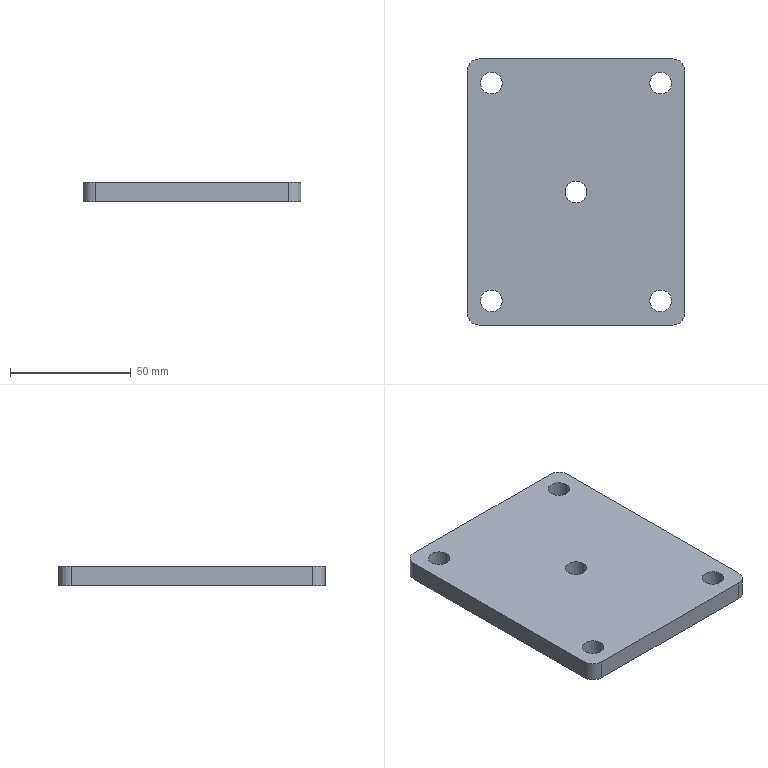Part | SolidWorks | features 3DProfileFeature 1, Extrusion 1, HoleWzd 1 | 1 solid | 20 faces | box 90 x 110 x 8 mm | volume 76484 mm3 | cylinder 14 | plane 6 | commonest cylinder face diameters 9 x10 10 x4
STEP:
#1=CARTESIAN_POINT('',(40.5,-35.,0.));
#2=VERTEX_POINT('',#1);
#3=CARTESIAN_POINT('',(49.5,-35.,0.));
#4=VERTEX_POINT('',#3);
#5=CARTESIAN_POINT('',(45.,-35.,0.));
#6=DIRECTION('',(0.,0.,1.));
#7=DIRECTION('',(1.,0.,0.));
#8=AXIS2_PLACEMENT_3D('',#5,#6,#7);
#9=CIRCLE('',#8,4.5);
#10=EDGE_CURVE('',#2,#4,#9,.T.);
#11=ORIENTED_EDGE('',*,*,#10,.F.);
#12=CARTESIAN_POINT('',(40.5,-35.,8.));
#13=VERTEX_POINT('',#12);
#14=CARTESIAN_POINT('',(40.5,-35.,8.));
#15=DIRECTION('',(0.,0.,1.));
#16=VECTOR('',#15,1000.);
#17=LINE('',#14,#16);
#18=EDGE_CURVE('',#2,#13,#17,.T.);
#19=ORIENTED_EDGE('',*,*,#18,.T.);
#20=CARTESIAN_POINT('',(49.5,-35.,8.));
#21=VERTEX_POINT('',#20);
#22=CARTESIAN_POINT('',(45.,-35.,8.));
#23=DIRECTION('',(0.,0.,1.));
#24=DIRECTION('',(1.,0.,0.));
#25=AXIS2_PLACEMENT_3D('',#22,#23,#24);
#26=CIRCLE('',#25,4.5);
#27=EDGE_CURVE('',#13,#21,#26,.T.);
#28=ORIENTED_EDGE('',*,*,#27,.T.);
#29=CARTESIAN_POINT('',(49.5,-35.,8.));
#30=DIRECTION('',(0.,0.,1.));
#31=VECTOR('',#30,1000.);
#32=LINE('',#29,#31);
#33=EDGE_CURVE('',#4,#21,#32,.T.);
#34=ORIENTED_EDGE('',*,*,#33,.F.);
#35=EDGE_LOOP('',(#11,#19,#28,#34));
#36=FACE_OUTER_BOUND('',#35,.T.);
#37=CARTESIAN_POINT('',(45.,-35.,8.));
#38=DIRECTION('',(0.,0.,1.));
#39=DIRECTION('',(1.,0.,0.));
#40=AXIS2_PLACEMENT_3D('',#37,#38,#39);
#41=CYLINDRICAL_SURFACE('',#40,4.5);
#42=ADVANCED_FACE('',(#36),#41,.F.);
#43=CARTESIAN_POINT('',(75.5,-80.,8.));
#44=VERTEX_POINT('',#43);
#45=CARTESIAN_POINT('',(84.5,-80.,8.));
#46=VERTEX_POINT('',#45);
#47=CARTESIAN_POINT('',(80.,-80.,8.));
#48=DIRECTION('',(0.,0.,1.));
#49=DIRECTION('',(1.,0.,0.));
#50=AXIS2_PLACEMENT_3D('',#47,#48,#49);
#51=CIRCLE('',#50,4.5);
#52=EDGE_CURVE('',#44,#46,#51,.T.);
#53=ORIENTED_EDGE('',*,*,#52,.T.);
#54=CARTESIAN_POINT('',(84.5,-80.,0.));
#55=VERTEX_POINT('',#54);
#56=CARTESIAN_POINT('',(84.5,-80.,8.));
#57=DIRECTION('',(0.,0.,-1.));
#58=VECTOR('',#57,1000.);
#59=LINE('',#56,#58);
#60=EDGE_CURVE('',#46,#55,#59,.T.);
#61=ORIENTED_EDGE('',*,*,#60,.T.);
#62=CARTESIAN_POINT('',(75.5,-80.,0.));
#63=VERTEX_POINT('',#62);
#64=CARTESIAN_POINT('',(80.,-80.,0.));
#65=DIRECTION('',(0.,0.,1.));
#66=DIRECTION('',(1.,0.,0.));
#67=AXIS2_PLACEMENT_3D('',#64,#65,#66);
#68=CIRCLE('',#67,4.5);
#69=EDGE_CURVE('',#63,#55,#68,.T.);
#70=ORIENTED_EDGE('',*,*,#69,.F.);
#71=CARTESIAN_POINT('',(75.5,-80.,8.));
#72=DIRECTION('',(0.,0.,-1.));
#73=VECTOR('',#72,1000.);
#74=LINE('',#71,#73);
#75=EDGE_CURVE('',#44,#63,#74,.T.);
#76=ORIENTED_EDGE('',*,*,#75,.F.);
#77=EDGE_LOOP('',(#53,#61,#70,#76));
#78=FACE_OUTER_BOUND('',#77,.T.);
#79=CARTESIAN_POINT('',(80.,-80.,8.));
#80=DIRECTION('',(0.,0.,-1.));
#81=DIRECTION('',(-1.,0.,0.));
#82=AXIS2_PLACEMENT_3D('',#79,#80,#81);
#83=CYLINDRICAL_SURFACE('',#82,4.5);
#84=ADVANCED_FACE('',(#78),#83,.F.);
#85=CARTESIAN_POINT('',(5.5,-80.,8.));
#86=VERTEX_POINT('',#85);
#87=CARTESIAN_POINT('',(14.5,-80.,8.));
#88=VERTEX_POINT('',#87);
#89=CARTESIAN_POINT('',(10.,-80.,8.));
#90=DIRECTION('',(0.,0.,1.));
#91=DIRECTION('',(1.,0.,0.));
#92=AXIS2_PLACEMENT_3D('',#89,#90,#91);
#93=CIRCLE('',#92,4.5);
#94=EDGE_CURVE('',#86,#88,#93,.T.);
#95=ORIENTED_EDGE('',*,*,#94,.T.);
#96=CARTESIAN_POINT('',(14.5,-80.,0.));
#97=VERTEX_POINT('',#96);
#98=CARTESIAN_POINT('',(14.5,-80.,8.));
#99=DIRECTION('',(0.,0.,-1.));
#100=VECTOR('',#99,1000.);
#101=LINE('',#98,#100);
#102=EDGE_CURVE('',#88,#97,#101,.T.);
#103=ORIENTED_EDGE('',*,*,#102,.T.);
#104=CARTESIAN_POINT('',(5.5,-80.,0.));
#105=VERTEX_POINT('',#104);
#106=CARTESIAN_POINT('',(10.,-80.,0.));
#107=DIRECTION('',(0.,0.,1.));
#108=DIRECTION('',(1.,0.,0.));
#109=AXIS2_PLACEMENT_3D('',#106,#107,#108);
#110=CIRCLE('',#109,4.5);
#111=EDGE_CURVE('',#105,#97,#110,.T.);
#112=ORIENTED_EDGE('',*,*,#111,.F.);
#113=CARTESIAN_POINT('',(5.5,-80.,8.));
#114=DIRECTION('',(0.,0.,-1.));
#115=VECTOR('',#114,1000.);
#116=LINE('',#113,#115);
#117=EDGE_CURVE('',#86,#105,#116,.T.);
#118=ORIENTED_EDGE('',*,*,#117,.F.);
#119=EDGE_LOOP('',(#95,#103,#112,#118));
#120=FACE_OUTER_BOUND('',#119,.T.);
#121=CARTESIAN_POINT('',(10.,-80.,8.));
#122=DIRECTION('',(0.,0.,-1.));
#123=DIRECTION('',(-1.,0.,0.));
#124=AXIS2_PLACEMENT_3D('',#121,#122,#123);
#125=CYLINDRICAL_SURFACE('',#124,4.5);
#126=ADVANCED_FACE('',(#120),#125,.F.);
#127=CARTESIAN_POINT('',(75.5,10.,8.));
#128=VERTEX_POINT('',#127);
#129=CARTESIAN_POINT('',(84.5,10.,8.));
#130=VERTEX_POINT('',#129);
#131=CARTESIAN_POINT('',(80.,10.,8.));
#132=DIRECTION('',(0.,0.,1.));
#133=DIRECTION('',(1.,0.,0.));
#134=AXIS2_PLACEMENT_3D('',#131,#132,#133);
#135=CIRCLE('',#134,4.5);
#136=EDGE_CURVE('',#128,#130,#135,.T.);
#137=ORIENTED_EDGE('',*,*,#136,.T.);
#138=CARTESIAN_POINT('',(84.5,10.,0.));
#139=VERTEX_POINT('',#138);
#140=CARTESIAN_POINT('',(84.5,10.,8.));
#141=DIRECTION('',(0.,0.,-1.));
#142=VECTOR('',#141,1000.);
#143=LINE('',#140,#142);
#144=EDGE_CURVE('',#130,#139,#143,.T.);
#145=ORIENTED_EDGE('',*,*,#144,.T.);
#146=CARTESIAN_POINT('',(75.5,10.,0.));
#147=VERTEX_POINT('',#146);
#148=CARTESIAN_POINT('',(80.,10.,0.));
#149=DIRECTION('',(0.,0.,1.));
#150=DIRECTION('',(1.,0.,0.));
#151=AXIS2_PLACEMENT_3D('',#148,#149,#150);
#152=CIRCLE('',#151,4.5);
#153=EDGE_CURVE('',#147,#139,#152,.T.);
#154=ORIENTED_EDGE('',*,*,#153,.F.);
#155=CARTESIAN_POINT('',(75.5,10.,8.));
#156=DIRECTION('',(0.,0.,-1.));
#157=VECTOR('',#156,1000.);
#158=LINE('',#155,#157);
#159=EDGE_CURVE('',#128,#147,#158,.T.);
#160=ORIENTED_EDGE('',*,*,#159,.F.);
#161=EDGE_LOOP('',(#137,#145,#154,#160));
#162=FACE_OUTER_BOUND('',#161,.T.);
#163=CARTESIAN_POINT('',(80.,10.,8.));
#164=DIRECTION('',(0.,0.,-1.));
#165=DIRECTION('',(-1.,0.,0.));
#166=AXIS2_PLACEMENT_3D('',#163,#164,#165);
#167=CYLINDRICAL_SURFACE('',#166,4.5);
#168=ADVANCED_FACE('',(#162),#167,.F.);
#169=CARTESIAN_POINT('',(5.5,10.,8.));
#170=VERTEX_POINT('',#169);
#171=CARTESIAN_POINT('',(14.5,10.,8.));
#172=VERTEX_POINT('',#171);
#173=CARTESIAN_POINT('',(10.,10.,8.));
#174=DIRECTION('',(0.,0.,1.));
#175=DIRECTION('',(1.,0.,0.));
#176=AXIS2_PLACEMENT_3D('',#173,#174,#175);
#177=CIRCLE('',#176,4.5);
#178=EDGE_CURVE('',#170,#172,#177,.T.);
#179=ORIENTED_EDGE('',*,*,#178,.T.);
#180=CARTESIAN_POINT('',(14.5,10.,0.));
#181=VERTEX_POINT('',#180);
#182=CARTESIAN_POINT('',(14.5,10.,8.));
#183=DIRECTION('',(0.,0.,-1.));
#184=VECTOR('',#183,1000.);
#185=LINE('',#182,#184);
#186=EDGE_CURVE('',#172,#181,#185,.T.);
#187=ORIENTED_EDGE('',*,*,#186,.T.);
#188=CARTESIAN_POINT('',(5.5,10.,0.));
#189=VERTEX_POINT('',#188);
#190=CARTESIAN_POINT('',(10.,10.,0.));
#191=DIRECTION('',(0.,0.,1.));
#192=DIRECTION('',(1.,0.,0.));
#193=AXIS2_PLACEMENT_3D('',#190,#191,#192);
#194=CIRCLE('',#193,4.5);
#195=EDGE_CURVE('',#189,#181,#194,.T.);
#196=ORIENTED_EDGE('',*,*,#195,.F.);
#197=CARTESIAN_POINT('',(5.5,10.,8.));
#198=DIRECTION('',(0.,0.,-1.));
#199=VECTOR('',#198,1000.);
#200=LINE('',#197,#199);
#201=EDGE_CURVE('',#170,#189,#200,.T.);
#202=ORIENTED_EDGE('',*,*,#201,.F.);
#203=EDGE_LOOP('',(#179,#187,#196,#202));
#204=FACE_OUTER_BOUND('',#203,.T.);
#205=CARTESIAN_POINT('',(10.,10.,8.));
#206=DIRECTION('',(0.,0.,-1.));
#207=DIRECTION('',(-1.,0.,0.));
#208=AXIS2_PLACEMENT_3D('',#205,#206,#207);
#209=CYLINDRICAL_SURFACE('',#208,4.5);
#210=ADVANCED_FACE('',(#204),#209,.F.);
#211=CARTESIAN_POINT('',(45.,-35.,8.));
#212=DIRECTION('',(0.,0.,1.));
#213=DIRECTION('',(1.,0.,0.));
#214=AXIS2_PLACEMENT_3D('',#211,#212,#213);
#215=CIRCLE('',#214,4.5);
#216=EDGE_CURVE('',#21,#13,#215,.T.);
#217=ORIENTED_EDGE('',*,*,#216,.F.);
#218=ORIENTED_EDGE('',*,*,#27,.F.);
#219=EDGE_LOOP('',(#217,#218));
#220=FACE_BOUND('',#219,.T.);
#221=ORIENTED_EDGE('',*,*,#94,.F.);
#222=CARTESIAN_POINT('',(10.,-80.,8.));
#223=DIRECTION('',(0.,0.,1.));
#224=DIRECTION('',(1.,0.,0.));
#225=AXIS2_PLACEMENT_3D('',#222,#223,#224);
#226=CIRCLE('',#225,4.5);
#227=EDGE_CURVE('',#88,#86,#226,.T.);
#228=ORIENTED_EDGE('',*,*,#227,.F.);
#229=EDGE_LOOP('',(#221,#228));
#230=FACE_BOUND('',#229,.T.);
#231=ORIENTED_EDGE('',*,*,#178,.F.);
#232=CARTESIAN_POINT('',(10.,10.,8.));
#233=DIRECTION('',(0.,0.,1.));
#234=DIRECTION('',(1.,0.,0.));
#235=AXIS2_PLACEMENT_3D('',#232,#233,#234);
#236=CIRCLE('',#235,4.5);
#237=EDGE_CURVE('',#172,#170,#236,.T.);
#238=ORIENTED_EDGE('',*,*,#237,.F.);
#239=EDGE_LOOP('',(#231,#238));
#240=FACE_BOUND('',#239,.T.);
#241=CARTESIAN_POINT('',(0.,-85.,8.));
#242=VERTEX_POINT('',#241);
#243=CARTESIAN_POINT('',(5.,-90.,8.));
#244=VERTEX_POINT('',#243);
#245=CARTESIAN_POINT('',(5.,-85.,8.));
#246=DIRECTION('',(0.,0.,1.));
#247=DIRECTION('',(1.,0.,0.));
#248=AXIS2_PLACEMENT_3D('',#245,#246,#247);
#249=CIRCLE('',#248,5.);
#250=EDGE_CURVE('',#242,#244,#249,.T.);
#251=ORIENTED_EDGE('',*,*,#250,.T.);
#252=CARTESIAN_POINT('',(85.,-90.,8.));
#253=VERTEX_POINT('',#252);
#254=CARTESIAN_POINT('',(5.,-90.,8.));
#255=DIRECTION('',(1.,0.,0.));
#256=VECTOR('',#255,1000.);
#257=LINE('',#254,#256);
#258=EDGE_CURVE('',#244,#253,#257,.T.);
#259=ORIENTED_EDGE('',*,*,#258,.T.);
#260=CARTESIAN_POINT('',(90.,-85.,8.));
#261=VERTEX_POINT('',#260);
#262=CARTESIAN_POINT('',(85.,-85.,8.));
#263=DIRECTION('',(0.,0.,1.));
#264=DIRECTION('',(-1.,0.,0.));
#265=AXIS2_PLACEMENT_3D('',#262,#263,#264);
#266=CIRCLE('',#265,5.);
#267=EDGE_CURVE('',#253,#261,#266,.T.);
#268=ORIENTED_EDGE('',*,*,#267,.T.);
#269=CARTESIAN_POINT('',(90.,15.,8.));
#270=VERTEX_POINT('',#269);
#271=CARTESIAN_POINT('',(90.,15.,8.));
#272=DIRECTION('',(0.,1.,0.));
#273=VECTOR('',#272,1000.);
#274=LINE('',#271,#273);
#275=EDGE_CURVE('',#261,#270,#274,.T.);
#276=ORIENTED_EDGE('',*,*,#275,.T.);
#277=CARTESIAN_POINT('',(85.,20.,8.));
#278=VERTEX_POINT('',#277);
#279=CARTESIAN_POINT('',(85.,15.,8.));
#280=DIRECTION('',(0.,0.,1.));
#281=DIRECTION('',(1.,0.,0.));
#282=AXIS2_PLACEMENT_3D('',#279,#280,#281);
#283=CIRCLE('',#282,5.);
#284=EDGE_CURVE('',#270,#278,#283,.T.);
#285=ORIENTED_EDGE('',*,*,#284,.T.);
#286=CARTESIAN_POINT('',(5.,20.,8.));
#287=VERTEX_POINT('',#286);
#288=CARTESIAN_POINT('',(5.,20.,8.));
#289=DIRECTION('',(-1.,0.,0.));
#290=VECTOR('',#289,1000.);
#291=LINE('',#288,#290);
#292=EDGE_CURVE('',#278,#287,#291,.T.);
#293=ORIENTED_EDGE('',*,*,#292,.T.);
#294=CARTESIAN_POINT('',(0.,15.,8.));
#295=VERTEX_POINT('',#294);
#296=CARTESIAN_POINT('',(5.,15.,8.));
#297=DIRECTION('',(0.,0.,1.));
#298=DIRECTION('',(1.,0.,0.));
#299=AXIS2_PLACEMENT_3D('',#296,#297,#298);
#300=CIRCLE('',#299,5.);
#301=EDGE_CURVE('',#287,#295,#300,.T.);
#302=ORIENTED_EDGE('',*,*,#301,.T.);
#303=CARTESIAN_POINT('',(0.,15.,8.));
#304=DIRECTION('',(0.,-1.,0.));
#305=VECTOR('',#304,1000.);
#306=LINE('',#303,#305);
#307=EDGE_CURVE('',#295,#242,#306,.T.);
#308=ORIENTED_EDGE('',*,*,#307,.T.);
#309=EDGE_LOOP('',(#251,#259,#268,#276,#285,#293,#302,#308));
#310=FACE_OUTER_BOUND('',#309,.T.);
#311=ORIENTED_EDGE('',*,*,#136,.F.);
#312=CARTESIAN_POINT('',(80.,10.,8.));
#313=DIRECTION('',(0.,0.,1.));
#314=DIRECTION('',(1.,0.,0.));
#315=AXIS2_PLACEMENT_3D('',#312,#313,#314);
#316=CIRCLE('',#315,4.5);
#317=EDGE_CURVE('',#130,#128,#316,.T.);
#318=ORIENTED_EDGE('',*,*,#317,.F.);
#319=EDGE_LOOP('',(#311,#318));
#320=FACE_BOUND('',#319,.T.);
#321=ORIENTED_EDGE('',*,*,#52,.F.);
#322=CARTESIAN_POINT('',(80.,-80.,8.));
#323=DIRECTION('',(0.,0.,1.));
#324=DIRECTION('',(1.,0.,0.));
#325=AXIS2_PLACEMENT_3D('',#322,#323,#324);
#326=CIRCLE('',#325,4.5);
#327=EDGE_CURVE('',#46,#44,#326,.T.);
#328=ORIENTED_EDGE('',*,*,#327,.F.);
#329=EDGE_LOOP('',(#321,#328));
#330=FACE_BOUND('',#329,.T.);
#331=CARTESIAN_POINT('',(5.,-85.,8.));
#332=DIRECTION('',(0.,0.,1.));
#333=DIRECTION('',(1.,0.,0.));
#334=AXIS2_PLACEMENT_3D('',#331,#332,#333);
#335=PLANE('',#334);
#336=ADVANCED_FACE('',(#220,#230,#240,#310,#320,#330),#335,.T.);
#337=CARTESIAN_POINT('',(45.,-35.,0.));
#338=DIRECTION('',(0.,0.,1.));
#339=DIRECTION('',(1.,0.,0.));
#340=AXIS2_PLACEMENT_3D('',#337,#338,#339);
#341=CIRCLE('',#340,4.5);
#342=EDGE_CURVE('',#4,#2,#341,.T.);
#343=ORIENTED_EDGE('',*,*,#342,.T.);
#344=ORIENTED_EDGE('',*,*,#10,.T.);
#345=EDGE_LOOP('',(#343,#344));
#346=FACE_BOUND('',#345,.T.);
#347=CARTESIAN_POINT('',(0.,-85.,0.));
#348=VERTEX_POINT('',#347);
#349=CARTESIAN_POINT('',(5.,-90.,0.));
#350=VERTEX_POINT('',#349);
#351=CARTESIAN_POINT('',(5.,-85.,0.));
#352=DIRECTION('',(0.,0.,1.));
#353=DIRECTION('',(1.,0.,0.));
#354=AXIS2_PLACEMENT_3D('',#351,#352,#353);
#355=CIRCLE('',#354,5.);
#356=EDGE_CURVE('',#348,#350,#355,.T.);
#357=ORIENTED_EDGE('',*,*,#356,.F.);
#358=CARTESIAN_POINT('',(0.,15.,0.));
#359=VERTEX_POINT('',#358);
#360=CARTESIAN_POINT('',(0.,15.,0.));
#361=DIRECTION('',(0.,-1.,0.));
#362=VECTOR('',#361,1000.);
#363=LINE('',#360,#362);
#364=EDGE_CURVE('',#359,#348,#363,.T.);
#365=ORIENTED_EDGE('',*,*,#364,.F.);
#366=CARTESIAN_POINT('',(5.,20.,0.));
#367=VERTEX_POINT('',#366);
#368=CARTESIAN_POINT('',(5.,15.,0.));
#369=DIRECTION('',(0.,0.,1.));
#370=DIRECTION('',(1.,0.,0.));
#371=AXIS2_PLACEMENT_3D('',#368,#369,#370);
#372=CIRCLE('',#371,5.);
#373=EDGE_CURVE('',#367,#359,#372,.T.);
#374=ORIENTED_EDGE('',*,*,#373,.F.);
#375=CARTESIAN_POINT('',(85.,20.,0.));
#376=VERTEX_POINT('',#375);
#377=CARTESIAN_POINT('',(5.,20.,0.));
#378=DIRECTION('',(-1.,0.,0.));
#379=VECTOR('',#378,1000.);
#380=LINE('',#377,#379);
#381=EDGE_CURVE('',#376,#367,#380,.T.);
#382=ORIENTED_EDGE('',*,*,#381,.F.);
#383=CARTESIAN_POINT('',(90.,15.,0.));
#384=VERTEX_POINT('',#383);
#385=CARTESIAN_POINT('',(85.,15.,0.));
#386=DIRECTION('',(0.,0.,1.));
#387=DIRECTION('',(1.,0.,0.));
#388=AXIS2_PLACEMENT_3D('',#385,#386,#387);
#389=CIRCLE('',#388,5.);
#390=EDGE_CURVE('',#384,#376,#389,.T.);
#391=ORIENTED_EDGE('',*,*,#390,.F.);
#392=CARTESIAN_POINT('',(90.,-85.,0.));
#393=VERTEX_POINT('',#392);
#394=CARTESIAN_POINT('',(90.,15.,0.));
#395=DIRECTION('',(0.,1.,0.));
#396=VECTOR('',#395,1000.);
#397=LINE('',#394,#396);
#398=EDGE_CURVE('',#393,#384,#397,.T.);
#399=ORIENTED_EDGE('',*,*,#398,.F.);
#400=CARTESIAN_POINT('',(85.,-90.,0.));
#401=VERTEX_POINT('',#400);
#402=CARTESIAN_POINT('',(85.,-85.,0.));
#403=DIRECTION('',(0.,0.,1.));
#404=DIRECTION('',(-1.,0.,0.));
#405=AXIS2_PLACEMENT_3D('',#402,#403,#404);
#406=CIRCLE('',#405,5.);
#407=EDGE_CURVE('',#401,#393,#406,.T.);
#408=ORIENTED_EDGE('',*,*,#407,.F.);
#409=CARTESIAN_POINT('',(5.,-90.,0.));
#410=DIRECTION('',(1.,0.,0.));
#411=VECTOR('',#410,1000.);
#412=LINE('',#409,#411);
#413=EDGE_CURVE('',#350,#401,#412,.T.);
#414=ORIENTED_EDGE('',*,*,#413,.F.);
#415=EDGE_LOOP('',(#357,#365,#374,#382,#391,#399,#408,#414));
#416=FACE_OUTER_BOUND('',#415,.T.);
#417=ORIENTED_EDGE('',*,*,#195,.T.);
#418=CARTESIAN_POINT('',(10.,10.,0.));
#419=DIRECTION('',(0.,0.,1.));
#420=DIRECTION('',(1.,0.,0.));
#421=AXIS2_PLACEMENT_3D('',#418,#419,#420);
#422=CIRCLE('',#421,4.5);
#423=EDGE_CURVE('',#181,#189,#422,.T.);
#424=ORIENTED_EDGE('',*,*,#423,.T.);
#425=EDGE_LOOP('',(#417,#424));
#426=FACE_BOUND('',#425,.T.);
#427=ORIENTED_EDGE('',*,*,#153,.T.);
#428=CARTESIAN_POINT('',(80.,10.,0.));
#429=DIRECTION('',(0.,0.,1.));
#430=DIRECTION('',(1.,0.,0.));
#431=AXIS2_PLACEMENT_3D('',#428,#429,#430);
#432=CIRCLE('',#431,4.5);
#433=EDGE_CURVE('',#139,#147,#432,.T.);
#434=ORIENTED_EDGE('',*,*,#433,.T.);
#435=EDGE_LOOP('',(#427,#434));
#436=FACE_BOUND('',#435,.T.);
#437=ORIENTED_EDGE('',*,*,#111,.T.);
#438=CARTESIAN_POINT('',(10.,-80.,0.));
#439=DIRECTION('',(0.,0.,1.));
#440=DIRECTION('',(1.,0.,0.));
#441=AXIS2_PLACEMENT_3D('',#438,#439,#440);
#442=CIRCLE('',#441,4.5);
#443=EDGE_CURVE('',#97,#105,#442,.T.);
#444=ORIENTED_EDGE('',*,*,#443,.T.);
#445=EDGE_LOOP('',(#437,#444));
#446=FACE_BOUND('',#445,.T.);
#447=ORIENTED_EDGE('',*,*,#69,.T.);
#448=CARTESIAN_POINT('',(80.,-80.,0.));
#449=DIRECTION('',(0.,0.,1.));
#450=DIRECTION('',(1.,0.,0.));
#451=AXIS2_PLACEMENT_3D('',#448,#449,#450);
#452=CIRCLE('',#451,4.5);
#453=EDGE_CURVE('',#55,#63,#452,.T.);
#454=ORIENTED_EDGE('',*,*,#453,.T.);
#455=EDGE_LOOP('',(#447,#454));
#456=FACE_BOUND('',#455,.T.);
#457=CARTESIAN_POINT('',(5.,-85.,0.));
#458=DIRECTION('',(0.,0.,1.));
#459=DIRECTION('',(1.,0.,0.));
#460=AXIS2_PLACEMENT_3D('',#457,#458,#459);
#461=PLANE('',#460);
#462=ADVANCED_FACE('',(#346,#416,#426,#436,#446,#456),#461,.F.);
#463=ORIENTED_EDGE('',*,*,#356,.T.);
#464=CARTESIAN_POINT('',(5.,-90.,8.));
#465=DIRECTION('',(0.,0.,-1.));
#466=VECTOR('',#465,1000.);
#467=LINE('',#464,#466);
#468=EDGE_CURVE('',#244,#350,#467,.T.);
#469=ORIENTED_EDGE('',*,*,#468,.F.);
#470=ORIENTED_EDGE('',*,*,#250,.F.);
#471=CARTESIAN_POINT('',(0.,-85.,8.));
#472=DIRECTION('',(0.,0.,-1.));
#473=VECTOR('',#472,1000.);
#474=LINE('',#471,#473);
#475=EDGE_CURVE('',#242,#348,#474,.T.);
#476=ORIENTED_EDGE('',*,*,#475,.T.);
#477=EDGE_LOOP('',(#463,#469,#470,#476));
#478=FACE_OUTER_BOUND('',#477,.T.);
#479=CARTESIAN_POINT('',(5.,-85.,8.));
#480=DIRECTION('',(0.,0.,-1.));
#481=DIRECTION('',(-1.,0.,0.));
#482=AXIS2_PLACEMENT_3D('',#479,#480,#481);
#483=CYLINDRICAL_SURFACE('',#482,5.);
#484=ADVANCED_FACE('',(#478),#483,.T.);
#485=ORIENTED_EDGE('',*,*,#413,.T.);
#486=CARTESIAN_POINT('',(85.,-90.,8.));
#487=DIRECTION('',(0.,0.,-1.));
#488=VECTOR('',#487,1000.);
#489=LINE('',#486,#488);
#490=EDGE_CURVE('',#253,#401,#489,.T.);
#491=ORIENTED_EDGE('',*,*,#490,.F.);
#492=ORIENTED_EDGE('',*,*,#258,.F.);
#493=ORIENTED_EDGE('',*,*,#468,.T.);
#494=EDGE_LOOP('',(#485,#491,#492,#493));
#495=FACE_OUTER_BOUND('',#494,.T.);
#496=CARTESIAN_POINT('',(5.,-90.,8.));
#497=DIRECTION('',(0.,1.,0.));
#498=DIRECTION('',(0.,0.,1.));
#499=AXIS2_PLACEMENT_3D('',#496,#497,#498);
#500=PLANE('',#499);
#501=ADVANCED_FACE('',(#495),#500,.F.);
#502=ORIENTED_EDGE('',*,*,#407,.T.);
#503=CARTESIAN_POINT('',(90.,-85.,8.));
#504=DIRECTION('',(0.,0.,-1.));
#505=VECTOR('',#504,1000.);
#506=LINE('',#503,#505);
#507=EDGE_CURVE('',#261,#393,#506,.T.);
#508=ORIENTED_EDGE('',*,*,#507,.F.);
#509=ORIENTED_EDGE('',*,*,#267,.F.);
#510=ORIENTED_EDGE('',*,*,#490,.T.);
#511=EDGE_LOOP('',(#502,#508,#509,#510));
#512=FACE_OUTER_BOUND('',#511,.T.);
#513=CARTESIAN_POINT('',(85.,-85.,8.));
#514=DIRECTION('',(0.,0.,-1.));
#515=DIRECTION('',(-1.,0.,0.));
#516=AXIS2_PLACEMENT_3D('',#513,#514,#515);
#517=CYLINDRICAL_SURFACE('',#516,5.);
#518=ADVANCED_FACE('',(#512),#517,.T.);
#519=ORIENTED_EDGE('',*,*,#398,.T.);
#520=CARTESIAN_POINT('',(90.,15.,8.));
#521=DIRECTION('',(0.,0.,-1.));
#522=VECTOR('',#521,1000.);
#523=LINE('',#520,#522);
#524=EDGE_CURVE('',#270,#384,#523,.T.);
#525=ORIENTED_EDGE('',*,*,#524,.F.);
#526=ORIENTED_EDGE('',*,*,#275,.F.);
#527=ORIENTED_EDGE('',*,*,#507,.T.);
#528=EDGE_LOOP('',(#519,#525,#526,#527));
#529=FACE_OUTER_BOUND('',#528,.T.);
#530=CARTESIAN_POINT('',(90.,15.,8.));
#531=DIRECTION('',(-1.,0.,0.));
#532=DIRECTION('',(0.,0.,1.));
#533=AXIS2_PLACEMENT_3D('',#530,#531,#532);
#534=PLANE('',#533);
#535=ADVANCED_FACE('',(#529),#534,.F.);
#536=ORIENTED_EDGE('',*,*,#390,.T.);
#537=CARTESIAN_POINT('',(85.,20.,8.));
#538=DIRECTION('',(0.,0.,-1.));
#539=VECTOR('',#538,1000.);
#540=LINE('',#537,#539);
#541=EDGE_CURVE('',#278,#376,#540,.T.);
#542=ORIENTED_EDGE('',*,*,#541,.F.);
#543=ORIENTED_EDGE('',*,*,#284,.F.);
#544=ORIENTED_EDGE('',*,*,#524,.T.);
#545=EDGE_LOOP('',(#536,#542,#543,#544));
#546=FACE_OUTER_BOUND('',#545,.T.);
#547=CARTESIAN_POINT('',(85.,15.,8.));
#548=DIRECTION('',(0.,0.,-1.));
#549=DIRECTION('',(-1.,0.,0.));
#550=AXIS2_PLACEMENT_3D('',#547,#548,#549);
#551=CYLINDRICAL_SURFACE('',#550,5.);
#552=ADVANCED_FACE('',(#546),#551,.T.);
#553=ORIENTED_EDGE('',*,*,#381,.T.);
#554=CARTESIAN_POINT('',(5.,20.,8.));
#555=DIRECTION('',(0.,0.,-1.));
#556=VECTOR('',#555,1000.);
#557=LINE('',#554,#556);
#558=EDGE_CURVE('',#287,#367,#557,.T.);
#559=ORIENTED_EDGE('',*,*,#558,.F.);
#560=ORIENTED_EDGE('',*,*,#292,.F.);
#561=ORIENTED_EDGE('',*,*,#541,.T.);
#562=EDGE_LOOP('',(#553,#559,#560,#561));
#563=FACE_OUTER_BOUND('',#562,.T.);
#564=CARTESIAN_POINT('',(5.,20.,8.));
#565=DIRECTION('',(0.,-1.,0.));
#566=DIRECTION('',(0.,0.,-1.));
#567=AXIS2_PLACEMENT_3D('',#564,#565,#566);
#568=PLANE('',#567);
#569=ADVANCED_FACE('',(#563),#568,.F.);
#570=ORIENTED_EDGE('',*,*,#373,.T.);
#571=CARTESIAN_POINT('',(0.,15.,8.));
#572=DIRECTION('',(0.,0.,-1.));
#573=VECTOR('',#572,1000.);
#574=LINE('',#571,#573);
#575=EDGE_CURVE('',#295,#359,#574,.T.);
#576=ORIENTED_EDGE('',*,*,#575,.F.);
#577=ORIENTED_EDGE('',*,*,#301,.F.);
#578=ORIENTED_EDGE('',*,*,#558,.T.);
#579=EDGE_LOOP('',(#570,#576,#577,#578));
#580=FACE_OUTER_BOUND('',#579,.T.);
#581=CARTESIAN_POINT('',(5.,15.,8.));
#582=DIRECTION('',(0.,0.,-1.));
#583=DIRECTION('',(-1.,0.,0.));
#584=AXIS2_PLACEMENT_3D('',#581,#582,#583);
#585=CYLINDRICAL_SURFACE('',#584,5.);
#586=ADVANCED_FACE('',(#580),#585,.T.);
#587=ORIENTED_EDGE('',*,*,#364,.T.);
#588=ORIENTED_EDGE('',*,*,#475,.F.);
#589=ORIENTED_EDGE('',*,*,#307,.F.);
#590=ORIENTED_EDGE('',*,*,#575,.T.);
#591=EDGE_LOOP('',(#587,#588,#589,#590));
#592=FACE_OUTER_BOUND('',#591,.T.);
#593=CARTESIAN_POINT('',(0.,15.,8.));
#594=DIRECTION('',(1.,0.,0.));
#595=DIRECTION('',(0.,1.,0.));
#596=AXIS2_PLACEMENT_3D('',#593,#594,#595);
#597=PLANE('',#596);
#598=ADVANCED_FACE('',(#592),#597,.F.);
#599=ORIENTED_EDGE('',*,*,#186,.F.);
#600=ORIENTED_EDGE('',*,*,#237,.T.);
#601=ORIENTED_EDGE('',*,*,#201,.T.);
#602=ORIENTED_EDGE('',*,*,#423,.F.);
#603=EDGE_LOOP('',(#599,#600,#601,#602));
#604=FACE_OUTER_BOUND('',#603,.T.);
#605=CARTESIAN_POINT('',(10.,10.,8.));
#606=DIRECTION('',(0.,0.,-1.));
#607=DIRECTION('',(-1.,0.,0.));
#608=AXIS2_PLACEMENT_3D('',#605,#606,#607);
#609=CYLINDRICAL_SURFACE('',#608,4.5);
#610=ADVANCED_FACE('',(#604),#609,.F.);
#611=ORIENTED_EDGE('',*,*,#144,.F.);
#612=ORIENTED_EDGE('',*,*,#317,.T.);
#613=ORIENTED_EDGE('',*,*,#159,.T.);
#614=ORIENTED_EDGE('',*,*,#433,.F.);
#615=EDGE_LOOP('',(#611,#612,#613,#614));
#616=FACE_OUTER_BOUND('',#615,.T.);
#617=CARTESIAN_POINT('',(80.,10.,8.));
#618=DIRECTION('',(0.,0.,-1.));
#619=DIRECTION('',(-1.,0.,0.));
#620=AXIS2_PLACEMENT_3D('',#617,#618,#619);
#621=CYLINDRICAL_SURFACE('',#620,4.5);
#622=ADVANCED_FACE('',(#616),#621,.F.);
#623=ORIENTED_EDGE('',*,*,#102,.F.);
#624=ORIENTED_EDGE('',*,*,#227,.T.);
#625=ORIENTED_EDGE('',*,*,#117,.T.);
#626=ORIENTED_EDGE('',*,*,#443,.F.);
#627=EDGE_LOOP('',(#623,#624,#625,#626));
#628=FACE_OUTER_BOUND('',#627,.T.);
#629=CARTESIAN_POINT('',(10.,-80.,8.));
#630=DIRECTION('',(0.,0.,-1.));
#631=DIRECTION('',(-1.,0.,0.));
#632=AXIS2_PLACEMENT_3D('',#629,#630,#631);
#633=CYLINDRICAL_SURFACE('',#632,4.5);
#634=ADVANCED_FACE('',(#628),#633,.F.);
#635=ORIENTED_EDGE('',*,*,#60,.F.);
#636=ORIENTED_EDGE('',*,*,#327,.T.);
#637=ORIENTED_EDGE('',*,*,#75,.T.);
#638=ORIENTED_EDGE('',*,*,#453,.F.);
#639=EDGE_LOOP('',(#635,#636,#637,#638));
#640=FACE_OUTER_BOUND('',#639,.T.);
#641=CARTESIAN_POINT('',(80.,-80.,8.));
#642=DIRECTION('',(0.,0.,-1.));
#643=DIRECTION('',(-1.,0.,0.));
#644=AXIS2_PLACEMENT_3D('',#641,#642,#643);
#645=CYLINDRICAL_SURFACE('',#644,4.5);
#646=ADVANCED_FACE('',(#640),#645,.F.);
#647=ORIENTED_EDGE('',*,*,#18,.F.);
#648=ORIENTED_EDGE('',*,*,#342,.F.);
#649=ORIENTED_EDGE('',*,*,#33,.T.);
#650=ORIENTED_EDGE('',*,*,#216,.T.);
#651=EDGE_LOOP('',(#647,#648,#649,#650));
#652=FACE_OUTER_BOUND('',#651,.T.);
#653=CARTESIAN_POINT('',(45.,-35.,8.));
#654=DIRECTION('',(0.,0.,1.));
#655=DIRECTION('',(1.,0.,0.));
#656=AXIS2_PLACEMENT_3D('',#653,#654,#655);
#657=CYLINDRICAL_SURFACE('',#656,4.5);
#658=ADVANCED_FACE('',(#652),#657,.F.);
#659=CLOSED_SHELL('',(#42,#84,#126,#168,#210,#336,#462,#484,#501,#518,#535,#552,#569,#586,#598,#610,#622,#634,#646,#658));
#660=MANIFOLD_SOLID_BREP('',#659);
#661=CARTESIAN_POINT('',(0.,0.,0.));
#662=DIRECTION('',(0.,0.,1.));
#663=DIRECTION('',(1.,0.,0.));
#664=AXIS2_PLACEMENT_3D('',#661,#662,#663);
#665=(LENGTH_UNIT()NAMED_UNIT(*)SI_UNIT(.MILLI.,.METRE.));
#666=UNCERTAINTY_MEASURE_WITH_UNIT(LENGTH_MEASURE(0.00001),#665,'','');
#667=(NAMED_UNIT(*)PLANE_ANGLE_UNIT()SI_UNIT($,.RADIAN.));
#668=(NAMED_UNIT(*)SI_UNIT($,.STERADIAN.)SOLID_ANGLE_UNIT());
#669=(GEOMETRIC_REPRESENTATION_CONTEXT(3)GLOBAL_UNCERTAINTY_ASSIGNED_CONTEXT((#666))GLOBAL_UNIT_ASSIGNED_CONTEXT((#665,#667,#668))REPRESENTATION_CONTEXT('',''));
#670=ADVANCED_BREP_SHAPE_REPRESENTATION('',(#660,#664),#669);